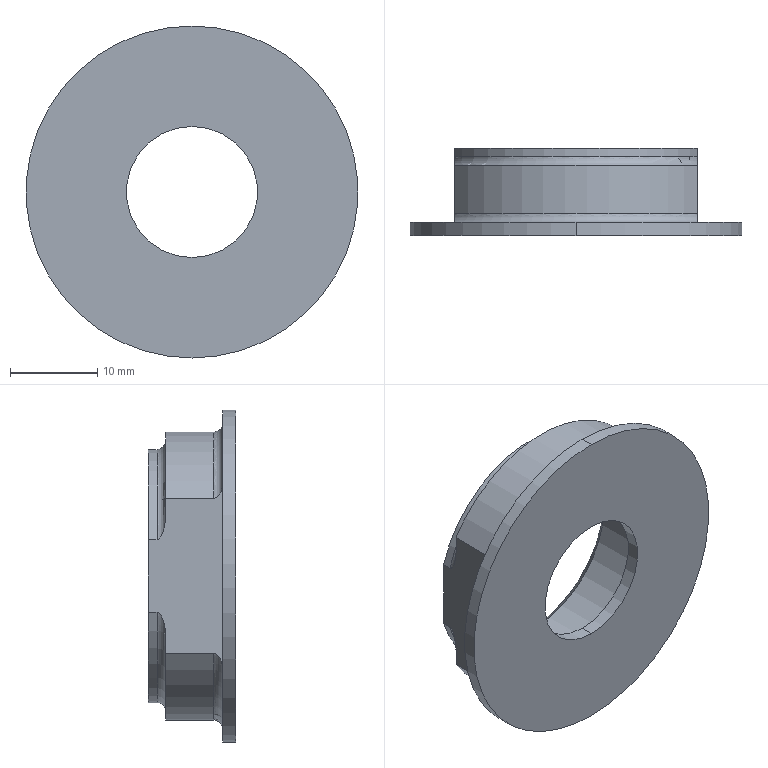Part | SolidWorks | features HoleWzd 1, ICE 1, Revolution 1 | 1 solid | 31 faces | box 38 x 10 x 38 mm | volume 4506 mm3 | cylinder 14 | plane 9 | torus 6 | cone 2 | commonest cylinder face diameters 29 x3 33 x3 15 x2 22 x2 26 x2 38 x2
STEP:
#1=CARTESIAN_POINT('',(0.,8.975,-11.));
#2=VERTEX_POINT('',#1);
#3=CARTESIAN_POINT('',(0.,8.975,11.));
#4=VERTEX_POINT('',#3);
#5=CARTESIAN_POINT('',(0.,8.975,0.));
#6=DIRECTION('',(0.,1.,0.));
#7=DIRECTION('',(0.,0.,1.));
#8=AXIS2_PLACEMENT_3D('',#5,#6,#7);
#9=CIRCLE('',#8,11.);
#10=EDGE_CURVE('',#2,#4,#9,.T.);
#11=ORIENTED_EDGE('',*,*,#10,.F.);
#12=CARTESIAN_POINT('',(0.,10.,-12.025));
#13=VERTEX_POINT('',#12);
#14=CARTESIAN_POINT('',(0.,10.,-12.025));
#15=DIRECTION('',(0.,0.7071,-0.7071));
#16=VECTOR('',#15,1000.);
#17=LINE('',#14,#16);
#18=EDGE_CURVE('',#2,#13,#17,.T.);
#19=ORIENTED_EDGE('',*,*,#18,.T.);
#20=CARTESIAN_POINT('',(0.,10.,12.025));
#21=VERTEX_POINT('',#20);
#22=CARTESIAN_POINT('',(0.,10.,0.));
#23=DIRECTION('',(0.,1.,0.));
#24=DIRECTION('',(0.,0.,1.));
#25=AXIS2_PLACEMENT_3D('',#22,#23,#24);
#26=CIRCLE('',#25,12.025);
#27=EDGE_CURVE('',#13,#21,#26,.T.);
#28=ORIENTED_EDGE('',*,*,#27,.T.);
#29=CARTESIAN_POINT('',(0.,10.,12.025));
#30=DIRECTION('',(0.,0.7071,0.7071));
#31=VECTOR('',#30,1000.);
#32=LINE('',#29,#31);
#33=EDGE_CURVE('',#4,#21,#32,.T.);
#34=ORIENTED_EDGE('',*,*,#33,.F.);
#35=EDGE_LOOP('',(#11,#19,#28,#34));
#36=FACE_OUTER_BOUND('',#35,.T.);
#37=CARTESIAN_POINT('',(0.,10.,0.));
#38=DIRECTION('',(0.,1.,0.));
#39=DIRECTION('',(0.,0.,1.));
#40=AXIS2_PLACEMENT_3D('',#37,#38,#39);
#41=CONICAL_SURFACE('',#40,12.025,0.7854);
#42=ADVANCED_FACE('',(#36),#41,.F.);
#43=CARTESIAN_POINT('',(0.,2.5,11.));
#44=VERTEX_POINT('',#43);
#45=CARTESIAN_POINT('',(0.,2.5,-11.));
#46=VERTEX_POINT('',#45);
#47=CARTESIAN_POINT('',(0.,2.5,0.));
#48=DIRECTION('',(0.,-1.,0.));
#49=DIRECTION('',(0.,0.,-1.));
#50=AXIS2_PLACEMENT_3D('',#47,#48,#49);
#51=CIRCLE('',#50,11.);
#52=EDGE_CURVE('',#44,#46,#51,.T.);
#53=ORIENTED_EDGE('',*,*,#52,.T.);
#54=CARTESIAN_POINT('',(0.,10.,-11.));
#55=DIRECTION('',(0.,1.,0.));
#56=VECTOR('',#55,1000.);
#57=LINE('',#54,#56);
#58=EDGE_CURVE('',#46,#2,#57,.T.);
#59=ORIENTED_EDGE('',*,*,#58,.T.);
#60=ORIENTED_EDGE('',*,*,#10,.T.);
#61=CARTESIAN_POINT('',(0.,10.,11.));
#62=DIRECTION('',(0.,1.,0.));
#63=VECTOR('',#62,1000.);
#64=LINE('',#61,#63);
#65=EDGE_CURVE('',#44,#4,#64,.T.);
#66=ORIENTED_EDGE('',*,*,#65,.F.);
#67=EDGE_LOOP('',(#53,#59,#60,#66));
#68=FACE_OUTER_BOUND('',#67,.T.);
#69=CARTESIAN_POINT('',(0.,10.,0.));
#70=DIRECTION('',(0.,1.,0.));
#71=DIRECTION('',(0.,0.,1.));
#72=AXIS2_PLACEMENT_3D('',#69,#70,#71);
#73=CYLINDRICAL_SURFACE('',#72,11.);
#74=ADVANCED_FACE('',(#68),#73,.F.);
#75=CARTESIAN_POINT('',(0.,1.5,-19.));
#76=VERTEX_POINT('',#75);
#77=CARTESIAN_POINT('',(0.,1.5,19.));
#78=VERTEX_POINT('',#77);
#79=CARTESIAN_POINT('',(0.,1.5,0.));
#80=DIRECTION('',(0.,-1.,0.));
#81=DIRECTION('',(0.,0.,-1.));
#82=AXIS2_PLACEMENT_3D('',#79,#80,#81);
#83=CIRCLE('',#82,19.);
#84=EDGE_CURVE('',#76,#78,#83,.T.);
#85=ORIENTED_EDGE('',*,*,#84,.T.);
#86=CARTESIAN_POINT('',(0.,0.,19.));
#87=VERTEX_POINT('',#86);
#88=CARTESIAN_POINT('',(0.,0.,19.));
#89=DIRECTION('',(0.,-1.,0.));
#90=VECTOR('',#89,1000.);
#91=LINE('',#88,#90);
#92=EDGE_CURVE('',#78,#87,#91,.T.);
#93=ORIENTED_EDGE('',*,*,#92,.T.);
#94=CARTESIAN_POINT('',(0.,0.,-19.));
#95=VERTEX_POINT('',#94);
#96=CARTESIAN_POINT('',(0.,0.,0.));
#97=DIRECTION('',(0.,-1.,0.));
#98=DIRECTION('',(0.,0.,-1.));
#99=AXIS2_PLACEMENT_3D('',#96,#97,#98);
#100=CIRCLE('',#99,19.);
#101=EDGE_CURVE('',#95,#87,#100,.T.);
#102=ORIENTED_EDGE('',*,*,#101,.F.);
#103=CARTESIAN_POINT('',(0.,0.,-19.));
#104=DIRECTION('',(0.,-1.,0.));
#105=VECTOR('',#104,1000.);
#106=LINE('',#103,#105);
#107=EDGE_CURVE('',#76,#95,#106,.T.);
#108=ORIENTED_EDGE('',*,*,#107,.F.);
#109=EDGE_LOOP('',(#85,#93,#102,#108));
#110=FACE_OUTER_BOUND('',#109,.T.);
#111=CARTESIAN_POINT('',(0.,0.,0.));
#112=DIRECTION('',(0.,-1.,0.));
#113=DIRECTION('',(0.,0.,-1.));
#114=AXIS2_PLACEMENT_3D('',#111,#112,#113);
#115=CYLINDRICAL_SURFACE('',#114,19.);
#116=ADVANCED_FACE('',(#110),#115,.T.);
#117=CARTESIAN_POINT('',(0.,2.5,13.));
#118=VERTEX_POINT('',#117);
#119=CARTESIAN_POINT('',(0.,2.5,-13.));
#120=VERTEX_POINT('',#119);
#121=CARTESIAN_POINT('',(0.,2.5,0.));
#122=DIRECTION('',(0.,-1.,0.));
#123=DIRECTION('',(0.,0.,-1.));
#124=AXIS2_PLACEMENT_3D('',#121,#122,#123);
#125=CIRCLE('',#124,13.);
#126=EDGE_CURVE('',#118,#120,#125,.T.);
#127=ORIENTED_EDGE('',*,*,#126,.F.);
#128=CARTESIAN_POINT('',(0.,1.5,13.));
#129=VERTEX_POINT('',#128);
#130=CARTESIAN_POINT('',(0.,0.,13.));
#131=DIRECTION('',(0.,-1.,0.));
#132=VECTOR('',#131,1000.);
#133=LINE('',#130,#132);
#134=EDGE_CURVE('',#118,#129,#133,.T.);
#135=ORIENTED_EDGE('',*,*,#134,.T.);
#136=CARTESIAN_POINT('',(0.,1.5,-13.));
#137=VERTEX_POINT('',#136);
#138=CARTESIAN_POINT('',(0.,1.5,0.));
#139=DIRECTION('',(0.,-1.,0.));
#140=DIRECTION('',(0.,0.,-1.));
#141=AXIS2_PLACEMENT_3D('',#138,#139,#140);
#142=CIRCLE('',#141,13.);
#143=EDGE_CURVE('',#129,#137,#142,.T.);
#144=ORIENTED_EDGE('',*,*,#143,.T.);
#145=CARTESIAN_POINT('',(0.,0.,-13.));
#146=DIRECTION('',(0.,-1.,0.));
#147=VECTOR('',#146,1000.);
#148=LINE('',#145,#147);
#149=EDGE_CURVE('',#120,#137,#148,.T.);
#150=ORIENTED_EDGE('',*,*,#149,.F.);
#151=EDGE_LOOP('',(#127,#135,#144,#150));
#152=FACE_OUTER_BOUND('',#151,.T.);
#153=CARTESIAN_POINT('',(0.,0.,0.));
#154=DIRECTION('',(0.,-1.,0.));
#155=DIRECTION('',(0.,0.,-1.));
#156=AXIS2_PLACEMENT_3D('',#153,#154,#155);
#157=CYLINDRICAL_SURFACE('',#156,13.);
#158=ADVANCED_FACE('',(#152),#157,.F.);
#159=CARTESIAN_POINT('',(0.,1.5,7.5));
#160=VERTEX_POINT('',#159);
#161=CARTESIAN_POINT('',(0.,1.5,-7.5));
#162=VERTEX_POINT('',#161);
#163=CARTESIAN_POINT('',(0.,1.5,0.));
#164=DIRECTION('',(0.,-1.,0.));
#165=DIRECTION('',(0.,0.,-1.));
#166=AXIS2_PLACEMENT_3D('',#163,#164,#165);
#167=CIRCLE('',#166,7.5);
#168=EDGE_CURVE('',#160,#162,#167,.T.);
#169=ORIENTED_EDGE('',*,*,#168,.F.);
#170=CARTESIAN_POINT('',(0.,0.,7.5));
#171=VERTEX_POINT('',#170);
#172=CARTESIAN_POINT('',(0.,0.,7.5));
#173=DIRECTION('',(0.,-1.,0.));
#174=VECTOR('',#173,1000.);
#175=LINE('',#172,#174);
#176=EDGE_CURVE('',#160,#171,#175,.T.);
#177=ORIENTED_EDGE('',*,*,#176,.T.);
#178=CARTESIAN_POINT('',(0.,0.,-7.5));
#179=VERTEX_POINT('',#178);
#180=CARTESIAN_POINT('',(0.,0.,0.));
#181=DIRECTION('',(0.,-1.,0.));
#182=DIRECTION('',(0.,0.,-1.));
#183=AXIS2_PLACEMENT_3D('',#180,#181,#182);
#184=CIRCLE('',#183,7.5);
#185=EDGE_CURVE('',#171,#179,#184,.T.);
#186=ORIENTED_EDGE('',*,*,#185,.T.);
#187=CARTESIAN_POINT('',(0.,0.,-7.5));
#188=DIRECTION('',(0.,-1.,0.));
#189=VECTOR('',#188,1000.);
#190=LINE('',#187,#189);
#191=EDGE_CURVE('',#162,#179,#190,.T.);
#192=ORIENTED_EDGE('',*,*,#191,.F.);
#193=EDGE_LOOP('',(#169,#177,#186,#192));
#194=FACE_OUTER_BOUND('',#193,.T.);
#195=CARTESIAN_POINT('',(0.,0.,0.));
#196=DIRECTION('',(0.,-1.,0.));
#197=DIRECTION('',(0.,0.,-1.));
#198=AXIS2_PLACEMENT_3D('',#195,#196,#197);
#199=CYLINDRICAL_SURFACE('',#198,7.5);
#200=ADVANCED_FACE('',(#194),#199,.F.);
#201=CARTESIAN_POINT('',(0.,1.5,-17.5));
#202=VERTEX_POINT('',#201);
#203=CARTESIAN_POINT('',(13.9,1.5,-10.632));
#204=VERTEX_POINT('',#203);
#205=CARTESIAN_POINT('',(0.,1.5,0.));
#206=DIRECTION('',(0.,-1.,0.));
#207=DIRECTION('',(0.,0.,-1.));
#208=AXIS2_PLACEMENT_3D('',#205,#206,#207);
#209=CIRCLE('',#208,17.5);
#210=EDGE_CURVE('',#202,#204,#209,.T.);
#211=ORIENTED_EDGE('',*,*,#210,.F.);
#212=CARTESIAN_POINT('',(0.,2.5,-16.5));
#213=VERTEX_POINT('',#212);
#214=CARTESIAN_POINT('',(0.,2.5,-17.5));
#215=DIRECTION('',(-1.,0.,0.));
#216=DIRECTION('',(0.,0.,1.));
#217=AXIS2_PLACEMENT_3D('',#214,#215,#216);
#218=CIRCLE('',#217,1.);
#219=EDGE_CURVE('',#202,#213,#218,.T.);
#220=ORIENTED_EDGE('',*,*,#219,.T.);
#221=CARTESIAN_POINT('',(13.9,2.5,-8.89));
#222=VERTEX_POINT('',#221);
#223=CARTESIAN_POINT('',(0.,2.5,0.));
#224=DIRECTION('',(0.,-1.,0.));
#225=DIRECTION('',(0.,0.,-1.));
#226=AXIS2_PLACEMENT_3D('',#223,#224,#225);
#227=CIRCLE('',#226,16.5);
#228=EDGE_CURVE('',#213,#222,#227,.T.);
#229=ORIENTED_EDGE('',*,*,#228,.T.);
#230=CARTESIAN_POINT('',(13.9,2.5,-8.89));
#231=CARTESIAN_POINT('',(13.9,2.408,-8.89));
#232=CARTESIAN_POINT('',(13.9,2.318,-8.915));
#233=CARTESIAN_POINT('',(13.9,2.154,-8.998));
#234=CARTESIAN_POINT('',(13.9,2.081,-9.055));
#235=CARTESIAN_POINT('',(13.9,1.952,-9.184));
#236=CARTESIAN_POINT('',(13.9,1.896,-9.257));
#237=CARTESIAN_POINT('',(13.9,1.797,-9.41));
#238=CARTESIAN_POINT('',(13.9,1.755,-9.49));
#239=CARTESIAN_POINT('',(13.9,1.642,-9.739));
#240=CARTESIAN_POINT('',(13.9,1.589,-9.914));
#241=CARTESIAN_POINT('',(13.9,1.518,-10.268));
#242=CARTESIAN_POINT('',(13.9,1.5,-10.451));
#243=CARTESIAN_POINT('',(13.9,1.5,-10.632));
#244=B_SPLINE_CURVE_WITH_KNOTS('',3,(#230,#231,#232,#233,#234,#235,#236,#237,#238,#239,#240,#241,#242,#243),.UNSPECIFIED.,.F.,.F.,(4,2,2,2,2,2,4),(0.004753,0.005027,0.005301,0.005575,0.005849,0.006397,0.006945),.UNSPECIFIED.);
#245=EDGE_CURVE('',#222,#204,#244,.T.);
#246=ORIENTED_EDGE('',*,*,#245,.T.);
#247=EDGE_LOOP('',(#211,#220,#229,#246));
#248=FACE_OUTER_BOUND('',#247,.T.);
#249=CARTESIAN_POINT('',(0.,2.5,0.));
#250=DIRECTION('',(0.,-1.,0.));
#251=DIRECTION('',(0.,0.,-1.));
#252=AXIS2_PLACEMENT_3D('',#249,#250,#251);
#253=TOROIDAL_SURFACE('',#252,17.5,1.);
#254=ADVANCED_FACE('',(#248),#253,.F.);
#255=CARTESIAN_POINT('',(-13.9,8.,-8.89));
#256=VERTEX_POINT('',#255);
#257=CARTESIAN_POINT('',(0.,8.,-16.5));
#258=VERTEX_POINT('',#257);
#259=CARTESIAN_POINT('',(0.,8.,0.));
#260=DIRECTION('',(0.,-1.,0.));
#261=DIRECTION('',(0.,0.,-1.));
#262=AXIS2_PLACEMENT_3D('',#259,#260,#261);
#263=CIRCLE('',#262,16.5);
#264=EDGE_CURVE('',#256,#258,#263,.T.);
#265=ORIENTED_EDGE('',*,*,#264,.T.);
#266=CARTESIAN_POINT('',(0.,0.,-16.5));
#267=DIRECTION('',(0.,-1.,0.));
#268=VECTOR('',#267,1000.);
#269=LINE('',#266,#268);
#270=EDGE_CURVE('',#258,#213,#269,.T.);
#271=ORIENTED_EDGE('',*,*,#270,.T.);
#272=CARTESIAN_POINT('',(-13.9,2.5,-8.89));
#273=VERTEX_POINT('',#272);
#274=CARTESIAN_POINT('',(0.,2.5,0.));
#275=DIRECTION('',(0.,-1.,0.));
#276=DIRECTION('',(0.,0.,-1.));
#277=AXIS2_PLACEMENT_3D('',#274,#275,#276);
#278=CIRCLE('',#277,16.5);
#279=EDGE_CURVE('',#273,#213,#278,.T.);
#280=ORIENTED_EDGE('',*,*,#279,.F.);
#281=CARTESIAN_POINT('',(-13.9,0.,-8.89));
#282=DIRECTION('',(0.,1.,0.));
#283=VECTOR('',#282,1000.);
#284=LINE('',#281,#283);
#285=EDGE_CURVE('',#273,#256,#284,.T.);
#286=ORIENTED_EDGE('',*,*,#285,.T.);
#287=EDGE_LOOP('',(#265,#271,#280,#286));
#288=FACE_OUTER_BOUND('',#287,.T.);
#289=CARTESIAN_POINT('',(0.,0.,0.));
#290=DIRECTION('',(0.,-1.,0.));
#291=DIRECTION('',(0.,0.,-1.));
#292=AXIS2_PLACEMENT_3D('',#289,#290,#291);
#293=CYLINDRICAL_SURFACE('',#292,16.5);
#294=ADVANCED_FACE('',(#288),#293,.T.);
#295=CARTESIAN_POINT('',(0.,8.,-15.5));
#296=VERTEX_POINT('',#295);
#297=CARTESIAN_POINT('',(13.9,8.,-6.859));
#298=VERTEX_POINT('',#297);
#299=CARTESIAN_POINT('',(0.,8.,0.));
#300=DIRECTION('',(0.,-1.,0.));
#301=DIRECTION('',(0.,0.,-1.));
#302=AXIS2_PLACEMENT_3D('',#299,#300,#301);
#303=CIRCLE('',#302,15.5);
#304=EDGE_CURVE('',#296,#298,#303,.T.);
#305=ORIENTED_EDGE('',*,*,#304,.F.);
#306=CARTESIAN_POINT('',(0.,9.,-14.5));
#307=VERTEX_POINT('',#306);
#308=CARTESIAN_POINT('',(0.,9.,-15.5));
#309=DIRECTION('',(-1.,0.,0.));
#310=DIRECTION('',(0.,0.,1.));
#311=AXIS2_PLACEMENT_3D('',#308,#309,#310);
#312=CIRCLE('',#311,1.);
#313=EDGE_CURVE('',#296,#307,#312,.T.);
#314=ORIENTED_EDGE('',*,*,#313,.T.);
#315=CARTESIAN_POINT('',(13.9,9.,-4.128));
#316=VERTEX_POINT('',#315);
#317=CARTESIAN_POINT('',(0.,9.,0.));
#318=DIRECTION('',(0.,-1.,0.));
#319=DIRECTION('',(0.,0.,-1.));
#320=AXIS2_PLACEMENT_3D('',#317,#318,#319);
#321=CIRCLE('',#320,14.5);
#322=EDGE_CURVE('',#307,#316,#321,.T.);
#323=ORIENTED_EDGE('',*,*,#322,.T.);
#324=CARTESIAN_POINT('',(13.9,9.,-4.128));
#325=CARTESIAN_POINT('',(13.9,8.936,-4.128));
#326=CARTESIAN_POINT('',(13.9,8.872,-4.152));
#327=CARTESIAN_POINT('',(13.9,8.763,-4.222));
#328=CARTESIAN_POINT('',(13.9,8.716,-4.267));
#329=CARTESIAN_POINT('',(13.9,8.59,-4.413));
#330=CARTESIAN_POINT('',(13.9,8.525,-4.523));
#331=CARTESIAN_POINT('',(13.9,8.352,-4.868));
#332=CARTESIAN_POINT('',(13.9,8.271,-5.108));
#333=CARTESIAN_POINT('',(13.9,8.137,-5.597));
#334=CARTESIAN_POINT('',(13.9,8.087,-5.848));
#335=CARTESIAN_POINT('',(13.9,8.018,-6.352));
#336=CARTESIAN_POINT('',(13.9,8.,-6.605));
#337=CARTESIAN_POINT('',(13.9,8.,-6.859));
#338=B_SPLINE_CURVE_WITH_KNOTS('',3,(#324,#325,#326,#327,#328,#329,#330,#331,#332,#333,#334,#335,#336,#337),.UNSPECIFIED.,.F.,.F.,(4,2,2,2,2,2,4),(0.005884,0.006078,0.006271,0.006658,0.007432,0.008206,0.00898),.UNSPECIFIED.);
#339=EDGE_CURVE('',#316,#298,#338,.T.);
#340=ORIENTED_EDGE('',*,*,#339,.T.);
#341=EDGE_LOOP('',(#305,#314,#323,#340));
#342=FACE_OUTER_BOUND('',#341,.T.);
#343=CARTESIAN_POINT('',(0.,9.,0.));
#344=DIRECTION('',(0.,-1.,0.));
#345=DIRECTION('',(0.,0.,-1.));
#346=AXIS2_PLACEMENT_3D('',#343,#344,#345);
#347=TOROIDAL_SURFACE('',#346,15.5,1.);
#348=ADVANCED_FACE('',(#342),#347,.F.);
#349=CARTESIAN_POINT('',(-13.9,10.,-4.128));
#350=VERTEX_POINT('',#349);
#351=CARTESIAN_POINT('',(0.,10.,-14.5));
#352=VERTEX_POINT('',#351);
#353=CARTESIAN_POINT('',(0.,10.,0.));
#354=DIRECTION('',(0.,-1.,0.));
#355=DIRECTION('',(0.,0.,-1.));
#356=AXIS2_PLACEMENT_3D('',#353,#354,#355);
#357=CIRCLE('',#356,14.5);
#358=EDGE_CURVE('',#350,#352,#357,.T.);
#359=ORIENTED_EDGE('',*,*,#358,.T.);
#360=CARTESIAN_POINT('',(0.,0.,-14.5));
#361=DIRECTION('',(0.,-1.,0.));
#362=VECTOR('',#361,1000.);
#363=LINE('',#360,#362);
#364=EDGE_CURVE('',#352,#307,#363,.T.);
#365=ORIENTED_EDGE('',*,*,#364,.T.);
#366=CARTESIAN_POINT('',(-13.9,9.,-4.128));
#367=VERTEX_POINT('',#366);
#368=CARTESIAN_POINT('',(0.,9.,0.));
#369=DIRECTION('',(0.,-1.,0.));
#370=DIRECTION('',(0.,0.,-1.));
#371=AXIS2_PLACEMENT_3D('',#368,#369,#370);
#372=CIRCLE('',#371,14.5);
#373=EDGE_CURVE('',#367,#307,#372,.T.);
#374=ORIENTED_EDGE('',*,*,#373,.F.);
#375=CARTESIAN_POINT('',(-13.9,0.,-4.128));
#376=DIRECTION('',(0.,1.,0.));
#377=VECTOR('',#376,1000.);
#378=LINE('',#375,#377);
#379=EDGE_CURVE('',#367,#350,#378,.T.);
#380=ORIENTED_EDGE('',*,*,#379,.T.);
#381=EDGE_LOOP('',(#359,#365,#374,#380));
#382=FACE_OUTER_BOUND('',#381,.T.);
#383=CARTESIAN_POINT('',(0.,0.,0.));
#384=DIRECTION('',(0.,-1.,0.));
#385=DIRECTION('',(0.,0.,-1.));
#386=AXIS2_PLACEMENT_3D('',#383,#384,#385);
#387=CYLINDRICAL_SURFACE('',#386,14.5);
#388=ADVANCED_FACE('',(#382),#387,.T.);
#389=CARTESIAN_POINT('',(0.,10.,0.));
#390=DIRECTION('',(0.,1.,0.));
#391=DIRECTION('',(0.,0.,1.));
#392=AXIS2_PLACEMENT_3D('',#389,#390,#391);
#393=CIRCLE('',#392,12.025);
#394=EDGE_CURVE('',#21,#13,#393,.T.);
#395=ORIENTED_EDGE('',*,*,#394,.F.);
#396=ORIENTED_EDGE('',*,*,#27,.F.);
#397=EDGE_LOOP('',(#395,#396));
#398=FACE_BOUND('',#397,.T.);
#399=ORIENTED_EDGE('',*,*,#358,.F.);
#400=CARTESIAN_POINT('',(-13.9,10.,4.128));
#401=VERTEX_POINT('',#400);
#402=CARTESIAN_POINT('',(-13.9,10.,-28.312));
#403=DIRECTION('',(0.,0.,1.));
#404=VECTOR('',#403,1000.);
#405=LINE('',#402,#404);
#406=EDGE_CURVE('',#350,#401,#405,.T.);
#407=ORIENTED_EDGE('',*,*,#406,.T.);
#408=CARTESIAN_POINT('',(13.9,10.,4.128));
#409=VERTEX_POINT('',#408);
#410=CARTESIAN_POINT('',(0.,10.,0.));
#411=DIRECTION('',(0.,-1.,0.));
#412=DIRECTION('',(0.,0.,-1.));
#413=AXIS2_PLACEMENT_3D('',#410,#411,#412);
#414=CIRCLE('',#413,14.5);
#415=EDGE_CURVE('',#409,#401,#414,.T.);
#416=ORIENTED_EDGE('',*,*,#415,.F.);
#417=CARTESIAN_POINT('',(13.9,10.,-4.128));
#418=VERTEX_POINT('',#417);
#419=CARTESIAN_POINT('',(13.9,10.,-28.312));
#420=DIRECTION('',(0.,0.,-1.));
#421=VECTOR('',#420,1000.);
#422=LINE('',#419,#421);
#423=EDGE_CURVE('',#409,#418,#422,.T.);
#424=ORIENTED_EDGE('',*,*,#423,.T.);
#425=CARTESIAN_POINT('',(0.,10.,0.));
#426=DIRECTION('',(0.,-1.,0.));
#427=DIRECTION('',(0.,0.,-1.));
#428=AXIS2_PLACEMENT_3D('',#425,#426,#427);
#429=CIRCLE('',#428,14.5);
#430=EDGE_CURVE('',#352,#418,#429,.T.);
#431=ORIENTED_EDGE('',*,*,#430,.F.);
#432=EDGE_LOOP('',(#399,#407,#416,#424,#431));
#433=FACE_OUTER_BOUND('',#432,.T.);
#434=CARTESIAN_POINT('',(14.5,10.,0.));
#435=DIRECTION('',(0.,1.,0.));
#436=DIRECTION('',(0.,0.,1.));
#437=AXIS2_PLACEMENT_3D('',#434,#435,#436);
#438=PLANE('',#437);
#439=ADVANCED_FACE('',(#398,#433),#438,.T.);
#440=ORIENTED_EDGE('',*,*,#364,.F.);
#441=ORIENTED_EDGE('',*,*,#430,.T.);
#442=CARTESIAN_POINT('',(13.9,0.,-4.128));
#443=DIRECTION('',(0.,-1.,0.));
#444=VECTOR('',#443,1000.);
#445=LINE('',#442,#444);
#446=EDGE_CURVE('',#418,#316,#445,.T.);
#447=ORIENTED_EDGE('',*,*,#446,.T.);
#448=ORIENTED_EDGE('',*,*,#322,.F.);
#449=EDGE_LOOP('',(#440,#441,#447,#448));
#450=FACE_OUTER_BOUND('',#449,.T.);
#451=CARTESIAN_POINT('',(0.,0.,0.));
#452=DIRECTION('',(0.,-1.,0.));
#453=DIRECTION('',(0.,0.,-1.));
#454=AXIS2_PLACEMENT_3D('',#451,#452,#453);
#455=CYLINDRICAL_SURFACE('',#454,14.5);
#456=ADVANCED_FACE('',(#450),#455,.T.);
#457=ORIENTED_EDGE('',*,*,#415,.T.);
#458=CARTESIAN_POINT('',(-13.9,9.,4.128));
#459=VERTEX_POINT('',#458);
#460=CARTESIAN_POINT('',(-13.9,0.,4.128));
#461=DIRECTION('',(0.,-1.,0.));
#462=VECTOR('',#461,1000.);
#463=LINE('',#460,#462);
#464=EDGE_CURVE('',#401,#459,#463,.T.);
#465=ORIENTED_EDGE('',*,*,#464,.T.);
#466=CARTESIAN_POINT('',(13.9,9.,4.128));
#467=VERTEX_POINT('',#466);
#468=CARTESIAN_POINT('',(0.,9.,0.));
#469=DIRECTION('',(0.,-1.,0.));
#470=DIRECTION('',(0.,0.,-1.));
#471=AXIS2_PLACEMENT_3D('',#468,#469,#470);
#472=CIRCLE('',#471,14.5);
#473=EDGE_CURVE('',#467,#459,#472,.T.);
#474=ORIENTED_EDGE('',*,*,#473,.F.);
#475=CARTESIAN_POINT('',(13.9,0.,4.128));
#476=DIRECTION('',(0.,1.,0.));
#477=VECTOR('',#476,1000.);
#478=LINE('',#475,#477);
#479=EDGE_CURVE('',#467,#409,#478,.T.);
#480=ORIENTED_EDGE('',*,*,#479,.T.);
#481=EDGE_LOOP('',(#457,#465,#474,#480));
#482=FACE_OUTER_BOUND('',#481,.T.);
#483=CARTESIAN_POINT('',(0.,0.,0.));
#484=DIRECTION('',(0.,-1.,0.));
#485=DIRECTION('',(0.,0.,-1.));
#486=AXIS2_PLACEMENT_3D('',#483,#484,#485);
#487=CYLINDRICAL_SURFACE('',#486,14.5);
#488=ADVANCED_FACE('',(#482),#487,.T.);
#489=ORIENTED_EDGE('',*,*,#313,.F.);
#490=CARTESIAN_POINT('',(-13.9,8.,-6.859));
#491=VERTEX_POINT('',#490);
#492=CARTESIAN_POINT('',(0.,8.,0.));
#493=DIRECTION('',(0.,-1.,0.));
#494=DIRECTION('',(0.,0.,-1.));
#495=AXIS2_PLACEMENT_3D('',#492,#493,#494);
#496=CIRCLE('',#495,15.5);
#497=EDGE_CURVE('',#491,#296,#496,.T.);
#498=ORIENTED_EDGE('',*,*,#497,.F.);
#499=CARTESIAN_POINT('',(-13.9,8.,-6.859));
#500=CARTESIAN_POINT('',(-13.9,8.,-6.604));
#501=CARTESIAN_POINT('',(-13.9,8.019,-6.352));
#502=CARTESIAN_POINT('',(-13.9,8.087,-5.851));
#503=CARTESIAN_POINT('',(-13.9,8.136,-5.602));
#504=CARTESIAN_POINT('',(-13.9,8.27,-5.109));
#505=CARTESIAN_POINT('',(-13.9,8.353,-4.867));
#506=CARTESIAN_POINT('',(-13.9,8.524,-4.526));
#507=CARTESIAN_POINT('',(-13.9,8.59,-4.414));
#508=CARTESIAN_POINT('',(-13.9,8.716,-4.267));
#509=CARTESIAN_POINT('',(-13.9,8.763,-4.221));
#510=CARTESIAN_POINT('',(-13.9,8.871,-4.152));
#511=CARTESIAN_POINT('',(-13.9,8.935,-4.128));
#512=CARTESIAN_POINT('',(-13.9,9.,-4.128));
#513=B_SPLINE_CURVE_WITH_KNOTS('',3,(#499,#500,#501,#502,#503,#504,#505,#506,#507,#508,#509,#510,#511,#512),.UNSPECIFIED.,.F.,.F.,(4,2,2,2,2,2,4),(0.002134,0.002899,0.003665,0.004431,0.004813,0.005005,0.005196),.UNSPECIFIED.);
#514=EDGE_CURVE('',#491,#367,#513,.T.);
#515=ORIENTED_EDGE('',*,*,#514,.T.);
#516=ORIENTED_EDGE('',*,*,#373,.T.);
#517=EDGE_LOOP('',(#489,#498,#515,#516));
#518=FACE_OUTER_BOUND('',#517,.T.);
#519=CARTESIAN_POINT('',(0.,9.,0.));
#520=DIRECTION('',(0.,-1.,0.));
#521=DIRECTION('',(0.,0.,-1.));
#522=AXIS2_PLACEMENT_3D('',#519,#520,#521);
#523=TOROIDAL_SURFACE('',#522,15.5,1.);
#524=ADVANCED_FACE('',(#518),#523,.F.);
#525=ORIENTED_EDGE('',*,*,#473,.T.);
#526=CARTESIAN_POINT('',(-13.9,8.,6.859));
#527=VERTEX_POINT('',#526);
#528=CARTESIAN_POINT('',(-13.9,9.,4.128));
#529=CARTESIAN_POINT('',(-13.9,8.935,4.128));
#530=CARTESIAN_POINT('',(-13.9,8.872,4.152));
#531=CARTESIAN_POINT('',(-13.9,8.764,4.221));
#532=CARTESIAN_POINT('',(-13.9,8.716,4.267));
#533=CARTESIAN_POINT('',(-13.9,8.591,4.413));
#534=CARTESIAN_POINT('',(-13.9,8.525,4.525));
#535=CARTESIAN_POINT('',(-13.9,8.353,4.866));
#536=CARTESIAN_POINT('',(-13.9,8.27,5.11));
#537=CARTESIAN_POINT('',(-13.9,8.136,5.602));
#538=CARTESIAN_POINT('',(-13.9,8.087,5.85));
#539=CARTESIAN_POINT('',(-13.9,8.019,6.351));
#540=CARTESIAN_POINT('',(-13.9,8.,6.604));
#541=CARTESIAN_POINT('',(-13.9,8.,6.859));
#542=B_SPLINE_CURVE_WITH_KNOTS('',3,(#528,#529,#530,#531,#532,#533,#534,#535,#536,#537,#538,#539,#540,#541),.UNSPECIFIED.,.F.,.F.,(4,2,2,2,2,2,4),(0.0000023,0.0001952,0.000388,0.0007737,0.001545,0.002317,0.003088),.UNSPECIFIED.);
#543=EDGE_CURVE('',#459,#527,#542,.T.);
#544=ORIENTED_EDGE('',*,*,#543,.T.);
#545=CARTESIAN_POINT('',(13.9,8.,6.859));
#546=VERTEX_POINT('',#545);
#547=CARTESIAN_POINT('',(0.,8.,0.));
#548=DIRECTION('',(0.,-1.,0.));
#549=DIRECTION('',(0.,0.,-1.));
#550=AXIS2_PLACEMENT_3D('',#547,#548,#549);
#551=CIRCLE('',#550,15.5);
#552=EDGE_CURVE('',#546,#527,#551,.T.);
#553=ORIENTED_EDGE('',*,*,#552,.F.);
#554=CARTESIAN_POINT('',(13.9,8.,6.859));
#555=CARTESIAN_POINT('',(13.9,8.,6.604));
#556=CARTESIAN_POINT('',(13.9,8.019,6.348));
#557=CARTESIAN_POINT('',(13.9,8.087,5.846));
#558=CARTESIAN_POINT('',(13.9,8.137,5.599));
#559=CARTESIAN_POINT('',(13.9,8.269,5.112));
#560=CARTESIAN_POINT('',(13.9,8.351,4.871));
#561=CARTESIAN_POINT('',(13.9,8.525,4.525));
#562=CARTESIAN_POINT('',(13.9,8.591,4.413));
#563=CARTESIAN_POINT('',(13.9,8.716,4.268));
#564=CARTESIAN_POINT('',(13.9,8.762,4.223));
#565=CARTESIAN_POINT('',(13.9,8.871,4.152));
#566=CARTESIAN_POINT('',(13.9,8.934,4.128));
#567=CARTESIAN_POINT('',(13.9,9.,4.128));
#568=B_SPLINE_CURVE_WITH_KNOTS('',3,(#554,#555,#556,#557,#558,#559,#560,#561,#562,#563,#564,#565,#566,#567),.UNSPECIFIED.,.F.,.F.,(4,2,2,2,2,2,4),(0.008027,0.008796,0.009565,0.01033,0.01072,0.01091,0.0111),.UNSPECIFIED.);
#569=EDGE_CURVE('',#546,#467,#568,.T.);
#570=ORIENTED_EDGE('',*,*,#569,.T.);
#571=EDGE_LOOP('',(#525,#544,#553,#570));
#572=FACE_OUTER_BOUND('',#571,.T.);
#573=CARTESIAN_POINT('',(0.,9.,0.));
#574=DIRECTION('',(0.,-1.,0.));
#575=DIRECTION('',(0.,0.,-1.));
#576=AXIS2_PLACEMENT_3D('',#573,#574,#575);
#577=TOROIDAL_SURFACE('',#576,15.5,1.);
#578=ADVANCED_FACE('',(#572),#577,.F.);
#579=ORIENTED_EDGE('',*,*,#264,.F.);
#580=CARTESIAN_POINT('',(-13.9,8.,0.));
#581=DIRECTION('',(0.,0.,1.));
#582=VECTOR('',#581,1000.);
#583=LINE('',#580,#582);
#584=EDGE_CURVE('',#256,#491,#583,.T.);
#585=ORIENTED_EDGE('',*,*,#584,.T.);
#586=ORIENTED_EDGE('',*,*,#497,.T.);
#587=ORIENTED_EDGE('',*,*,#304,.T.);
#588=CARTESIAN_POINT('',(13.9,8.,-8.89));
#589=VERTEX_POINT('',#588);
#590=CARTESIAN_POINT('',(13.9,8.,0.));
#591=DIRECTION('',(0.,0.,-1.));
#592=VECTOR('',#591,1000.);
#593=LINE('',#590,#592);
#594=EDGE_CURVE('',#298,#589,#593,.T.);
#595=ORIENTED_EDGE('',*,*,#594,.T.);
#596=CARTESIAN_POINT('',(0.,8.,0.));
#597=DIRECTION('',(0.,-1.,0.));
#598=DIRECTION('',(0.,0.,-1.));
#599=AXIS2_PLACEMENT_3D('',#596,#597,#598);
#600=CIRCLE('',#599,16.5);
#601=EDGE_CURVE('',#258,#589,#600,.T.);
#602=ORIENTED_EDGE('',*,*,#601,.F.);
#603=EDGE_LOOP('',(#579,#585,#586,#587,#595,#602));
#604=FACE_OUTER_BOUND('',#603,.T.);
#605=CARTESIAN_POINT('',(15.5,8.,0.));
#606=DIRECTION('',(0.,1.,0.));
#607=DIRECTION('',(0.,0.,1.));
#608=AXIS2_PLACEMENT_3D('',#605,#606,#607);
#609=PLANE('',#608);
#610=ADVANCED_FACE('',(#604),#609,.T.);
#611=ORIENTED_EDGE('',*,*,#552,.T.);
#612=CARTESIAN_POINT('',(-13.9,8.,8.89));
#613=VERTEX_POINT('',#612);
#614=CARTESIAN_POINT('',(-13.9,8.,0.));
#615=DIRECTION('',(0.,0.,1.));
#616=VECTOR('',#615,1000.);
#617=LINE('',#614,#616);
#618=EDGE_CURVE('',#527,#613,#617,.T.);
#619=ORIENTED_EDGE('',*,*,#618,.T.);
#620=CARTESIAN_POINT('',(13.9,8.,8.89));
#621=VERTEX_POINT('',#620);
#622=CARTESIAN_POINT('',(0.,8.,0.));
#623=DIRECTION('',(0.,-1.,0.));
#624=DIRECTION('',(0.,0.,-1.));
#625=AXIS2_PLACEMENT_3D('',#622,#623,#624);
#626=CIRCLE('',#625,16.5);
#627=EDGE_CURVE('',#621,#613,#626,.T.);
#628=ORIENTED_EDGE('',*,*,#627,.F.);
#629=CARTESIAN_POINT('',(13.9,8.,0.));
#630=DIRECTION('',(0.,0.,-1.));
#631=VECTOR('',#630,1000.);
#632=LINE('',#629,#631);
#633=EDGE_CURVE('',#621,#546,#632,.T.);
#634=ORIENTED_EDGE('',*,*,#633,.T.);
#635=EDGE_LOOP('',(#611,#619,#628,#634));
#636=FACE_OUTER_BOUND('',#635,.T.);
#637=CARTESIAN_POINT('',(15.5,8.,0.));
#638=DIRECTION('',(0.,1.,0.));
#639=DIRECTION('',(0.,0.,1.));
#640=AXIS2_PLACEMENT_3D('',#637,#638,#639);
#641=PLANE('',#640);
#642=ADVANCED_FACE('',(#636),#641,.T.);
#643=ORIENTED_EDGE('',*,*,#270,.F.);
#644=ORIENTED_EDGE('',*,*,#601,.T.);
#645=CARTESIAN_POINT('',(13.9,0.,-8.89));
#646=DIRECTION('',(0.,-1.,0.));
#647=VECTOR('',#646,1000.);
#648=LINE('',#645,#647);
#649=EDGE_CURVE('',#589,#222,#648,.T.);
#650=ORIENTED_EDGE('',*,*,#649,.T.);
#651=ORIENTED_EDGE('',*,*,#228,.F.);
#652=EDGE_LOOP('',(#643,#644,#650,#651));
#653=FACE_OUTER_BOUND('',#652,.T.);
#654=CARTESIAN_POINT('',(0.,0.,0.));
#655=DIRECTION('',(0.,-1.,0.));
#656=DIRECTION('',(0.,0.,-1.));
#657=AXIS2_PLACEMENT_3D('',#654,#655,#656);
#658=CYLINDRICAL_SURFACE('',#657,16.5);
#659=ADVANCED_FACE('',(#653),#658,.T.);
#660=ORIENTED_EDGE('',*,*,#627,.T.);
#661=CARTESIAN_POINT('',(-13.9,2.5,8.89));
#662=VERTEX_POINT('',#661);
#663=CARTESIAN_POINT('',(-13.9,0.,8.89));
#664=DIRECTION('',(0.,-1.,0.));
#665=VECTOR('',#664,1000.);
#666=LINE('',#663,#665);
#667=EDGE_CURVE('',#613,#662,#666,.T.);
#668=ORIENTED_EDGE('',*,*,#667,.T.);
#669=CARTESIAN_POINT('',(13.9,2.5,8.89));
#670=VERTEX_POINT('',#669);
#671=CARTESIAN_POINT('',(0.,2.5,0.));
#672=DIRECTION('',(0.,-1.,0.));
#673=DIRECTION('',(0.,0.,-1.));
#674=AXIS2_PLACEMENT_3D('',#671,#672,#673);
#675=CIRCLE('',#674,16.5);
#676=EDGE_CURVE('',#670,#662,#675,.T.);
#677=ORIENTED_EDGE('',*,*,#676,.F.);
#678=CARTESIAN_POINT('',(13.9,0.,8.89));
#679=DIRECTION('',(0.,1.,0.));
#680=VECTOR('',#679,1000.);
#681=LINE('',#678,#680);
#682=EDGE_CURVE('',#670,#621,#681,.T.);
#683=ORIENTED_EDGE('',*,*,#682,.T.);
#684=EDGE_LOOP('',(#660,#668,#677,#683));
#685=FACE_OUTER_BOUND('',#684,.T.);
#686=CARTESIAN_POINT('',(0.,0.,0.));
#687=DIRECTION('',(0.,-1.,0.));
#688=DIRECTION('',(0.,0.,-1.));
#689=AXIS2_PLACEMENT_3D('',#686,#687,#688);
#690=CYLINDRICAL_SURFACE('',#689,16.5);
#691=ADVANCED_FACE('',(#685),#690,.T.);
#692=ORIENTED_EDGE('',*,*,#219,.F.);
#693=CARTESIAN_POINT('',(-13.9,1.5,-10.632));
#694=VERTEX_POINT('',#693);
#695=CARTESIAN_POINT('',(0.,1.5,0.));
#696=DIRECTION('',(0.,-1.,0.));
#697=DIRECTION('',(0.,0.,-1.));
#698=AXIS2_PLACEMENT_3D('',#695,#696,#697);
#699=CIRCLE('',#698,17.5);
#700=EDGE_CURVE('',#694,#202,#699,.T.);
#701=ORIENTED_EDGE('',*,*,#700,.F.);
#702=CARTESIAN_POINT('',(-13.9,1.5,-10.632));
#703=CARTESIAN_POINT('',(-13.9,1.5,-10.451));
#704=CARTESIAN_POINT('',(-13.9,1.518,-10.268));
#705=CARTESIAN_POINT('',(-13.9,1.589,-9.913));
#706=CARTESIAN_POINT('',(-13.9,1.642,-9.741));
#707=CARTESIAN_POINT('',(-13.9,1.791,-9.408));
#708=CARTESIAN_POINT('',(-13.9,1.889,-9.248));
#709=CARTESIAN_POINT('',(-13.9,2.081,-9.055));
#710=CARTESIAN_POINT('',(-13.9,2.153,-8.998));
#711=CARTESIAN_POINT('',(-13.9,2.318,-8.915));
#712=CARTESIAN_POINT('',(-13.9,2.409,-8.89));
#713=CARTESIAN_POINT('',(-13.9,2.5,-8.89));
#714=B_SPLINE_CURVE_WITH_KNOTS('',3,(#702,#703,#704,#705,#706,#707,#708,#709,#710,#711,#712,#713),.UNSPECIFIED.,.F.,.F.,(4,2,2,2,2,4),(0.001543,0.002087,0.002631,0.003175,0.003447,0.003719),.UNSPECIFIED.);
#715=EDGE_CURVE('',#694,#273,#714,.T.);
#716=ORIENTED_EDGE('',*,*,#715,.T.);
#717=ORIENTED_EDGE('',*,*,#279,.T.);
#718=EDGE_LOOP('',(#692,#701,#716,#717));
#719=FACE_OUTER_BOUND('',#718,.T.);
#720=CARTESIAN_POINT('',(0.,2.5,0.));
#721=DIRECTION('',(0.,-1.,0.));
#722=DIRECTION('',(0.,0.,-1.));
#723=AXIS2_PLACEMENT_3D('',#720,#721,#722);
#724=TOROIDAL_SURFACE('',#723,17.5,1.);
#725=ADVANCED_FACE('',(#719),#724,.F.);
#726=ORIENTED_EDGE('',*,*,#676,.T.);
#727=CARTESIAN_POINT('',(-13.9,1.5,10.632));
#728=VERTEX_POINT('',#727);
#729=CARTESIAN_POINT('',(-13.9,2.5,8.89));
#730=CARTESIAN_POINT('',(-13.9,2.408,8.89));
#731=CARTESIAN_POINT('',(-13.9,2.318,8.915));
#732=CARTESIAN_POINT('',(-13.9,2.154,8.998));
#733=CARTESIAN_POINT('',(-13.9,2.081,9.055));
#734=CARTESIAN_POINT('',(-13.9,1.888,9.249));
#735=CARTESIAN_POINT('',(-13.9,1.792,9.407));
#736=CARTESIAN_POINT('',(-13.9,1.642,9.74));
#737=CARTESIAN_POINT('',(-13.9,1.589,9.913));
#738=CARTESIAN_POINT('',(-13.9,1.518,10.268));
#739=CARTESIAN_POINT('',(-13.9,1.5,10.451));
#740=CARTESIAN_POINT('',(-13.9,1.5,10.632));
#741=B_SPLINE_CURVE_WITH_KNOTS('',3,(#729,#730,#731,#732,#733,#734,#735,#736,#737,#738,#739,#740),.UNSPECIFIED.,.F.,.F.,(4,2,2,2,2,4),(0.008397,0.00867,0.008943,0.00949,0.01004,0.01058),.UNSPECIFIED.);
#742=EDGE_CURVE('',#662,#728,#741,.T.);
#743=ORIENTED_EDGE('',*,*,#742,.T.);
#744=CARTESIAN_POINT('',(13.9,1.5,10.632));
#745=VERTEX_POINT('',#744);
#746=CARTESIAN_POINT('',(0.,1.5,0.));
#747=DIRECTION('',(0.,-1.,0.));
#748=DIRECTION('',(0.,0.,-1.));
#749=AXIS2_PLACEMENT_3D('',#746,#747,#748);
#750=CIRCLE('',#749,17.5);
#751=EDGE_CURVE('',#745,#728,#750,.T.);
#752=ORIENTED_EDGE('',*,*,#751,.F.);
#753=CARTESIAN_POINT('',(13.9,1.5,10.632));
#754=CARTESIAN_POINT('',(13.9,1.5,10.45));
#755=CARTESIAN_POINT('',(13.9,1.518,10.268));
#756=CARTESIAN_POINT('',(13.9,1.589,9.914));
#757=CARTESIAN_POINT('',(13.9,1.643,9.739));
#758=CARTESIAN_POINT('',(13.9,1.792,9.407));
#759=CARTESIAN_POINT('',(13.9,1.889,9.248));
#760=CARTESIAN_POINT('',(13.9,2.081,9.055));
#761=CARTESIAN_POINT('',(13.9,2.154,8.998));
#762=CARTESIAN_POINT('',(13.9,2.317,8.915));
#763=CARTESIAN_POINT('',(13.9,2.409,8.89));
#764=CARTESIAN_POINT('',(13.9,2.5,8.89));
#765=B_SPLINE_CURVE_WITH_KNOTS('',3,(#753,#754,#755,#756,#757,#758,#759,#760,#761,#762,#763,#764),.UNSPECIFIED.,.F.,.F.,(4,2,2,2,2,4),(0.00637,0.006915,0.007459,0.008004,0.008276,0.008548),.UNSPECIFIED.);
#766=EDGE_CURVE('',#745,#670,#765,.T.);
#767=ORIENTED_EDGE('',*,*,#766,.T.);
#768=EDGE_LOOP('',(#726,#743,#752,#767));
#769=FACE_OUTER_BOUND('',#768,.T.);
#770=CARTESIAN_POINT('',(0.,2.5,0.));
#771=DIRECTION('',(0.,-1.,0.));
#772=DIRECTION('',(0.,0.,-1.));
#773=AXIS2_PLACEMENT_3D('',#770,#771,#772);
#774=TOROIDAL_SURFACE('',#773,17.5,1.);
#775=ADVANCED_FACE('',(#769),#774,.F.);
#776=ORIENTED_EDGE('',*,*,#176,.F.);
#777=CARTESIAN_POINT('',(0.,1.5,0.));
#778=DIRECTION('',(0.,-1.,0.));
#779=DIRECTION('',(0.,0.,-1.));
#780=AXIS2_PLACEMENT_3D('',#777,#778,#779);
#781=CIRCLE('',#780,7.5);
#782=EDGE_CURVE('',#162,#160,#781,.T.);
#783=ORIENTED_EDGE('',*,*,#782,.F.);
#784=ORIENTED_EDGE('',*,*,#191,.T.);
#785=CARTESIAN_POINT('',(0.,0.,0.));
#786=DIRECTION('',(0.,-1.,0.));
#787=DIRECTION('',(0.,0.,-1.));
#788=AXIS2_PLACEMENT_3D('',#785,#786,#787);
#789=CIRCLE('',#788,7.5);
#790=EDGE_CURVE('',#179,#171,#789,.T.);
#791=ORIENTED_EDGE('',*,*,#790,.T.);
#792=EDGE_LOOP('',(#776,#783,#784,#791));
#793=FACE_OUTER_BOUND('',#792,.T.);
#794=CARTESIAN_POINT('',(0.,0.,0.));
#795=DIRECTION('',(0.,-1.,0.));
#796=DIRECTION('',(0.,0.,-1.));
#797=AXIS2_PLACEMENT_3D('',#794,#795,#796);
#798=CYLINDRICAL_SURFACE('',#797,7.5);
#799=ADVANCED_FACE('',(#793),#798,.F.);
#800=ORIENTED_EDGE('',*,*,#782,.T.);
#801=ORIENTED_EDGE('',*,*,#168,.T.);
#802=EDGE_LOOP('',(#800,#801));
#803=FACE_BOUND('',#802,.T.);
#804=CARTESIAN_POINT('',(0.,1.5,0.));
#805=DIRECTION('',(0.,-1.,0.));
#806=DIRECTION('',(0.,0.,-1.));
#807=AXIS2_PLACEMENT_3D('',#804,#805,#806);
#808=CIRCLE('',#807,13.);
#809=EDGE_CURVE('',#137,#129,#808,.T.);
#810=ORIENTED_EDGE('',*,*,#809,.F.);
#811=ORIENTED_EDGE('',*,*,#143,.F.);
#812=EDGE_LOOP('',(#810,#811));
#813=FACE_OUTER_BOUND('',#812,.T.);
#814=CARTESIAN_POINT('',(13.,1.5,0.));
#815=DIRECTION('',(0.,1.,0.));
#816=DIRECTION('',(0.,0.,1.));
#817=AXIS2_PLACEMENT_3D('',#814,#815,#816);
#818=PLANE('',#817);
#819=ADVANCED_FACE('',(#803,#813),#818,.T.);
#820=ORIENTED_EDGE('',*,*,#134,.F.);
#821=CARTESIAN_POINT('',(0.,2.5,0.));
#822=DIRECTION('',(0.,-1.,0.));
#823=DIRECTION('',(0.,0.,-1.));
#824=AXIS2_PLACEMENT_3D('',#821,#822,#823);
#825=CIRCLE('',#824,13.);
#826=EDGE_CURVE('',#120,#118,#825,.T.);
#827=ORIENTED_EDGE('',*,*,#826,.F.);
#828=ORIENTED_EDGE('',*,*,#149,.T.);
#829=ORIENTED_EDGE('',*,*,#809,.T.);
#830=EDGE_LOOP('',(#820,#827,#828,#829));
#831=FACE_OUTER_BOUND('',#830,.T.);
#832=CARTESIAN_POINT('',(0.,0.,0.));
#833=DIRECTION('',(0.,-1.,0.));
#834=DIRECTION('',(0.,0.,-1.));
#835=AXIS2_PLACEMENT_3D('',#832,#833,#834);
#836=CYLINDRICAL_SURFACE('',#835,13.);
#837=ADVANCED_FACE('',(#831),#836,.F.);
#838=ORIENTED_EDGE('',*,*,#52,.F.);
#839=CARTESIAN_POINT('',(0.,2.5,0.));
#840=DIRECTION('',(0.,-1.,0.));
#841=DIRECTION('',(0.,0.,-1.));
#842=AXIS2_PLACEMENT_3D('',#839,#840,#841);
#843=CIRCLE('',#842,11.);
#844=EDGE_CURVE('',#46,#44,#843,.T.);
#845=ORIENTED_EDGE('',*,*,#844,.F.);
#846=EDGE_LOOP('',(#838,#845));
#847=FACE_BOUND('',#846,.T.);
#848=ORIENTED_EDGE('',*,*,#826,.T.);
#849=ORIENTED_EDGE('',*,*,#126,.T.);
#850=EDGE_LOOP('',(#848,#849));
#851=FACE_OUTER_BOUND('',#850,.T.);
#852=CARTESIAN_POINT('',(10.,2.5,0.));
#853=DIRECTION('',(0.,-1.,0.));
#854=DIRECTION('',(0.,0.,-1.));
#855=AXIS2_PLACEMENT_3D('',#852,#853,#854);
#856=PLANE('',#855);
#857=ADVANCED_FACE('',(#847,#851),#856,.T.);
#858=ORIENTED_EDGE('',*,*,#751,.T.);
#859=CARTESIAN_POINT('',(-13.9,1.5,-28.312));
#860=DIRECTION('',(0.,0.,-1.));
#861=VECTOR('',#860,1000.);
#862=LINE('',#859,#861);
#863=EDGE_CURVE('',#728,#694,#862,.T.);
#864=ORIENTED_EDGE('',*,*,#863,.T.);
#865=ORIENTED_EDGE('',*,*,#700,.T.);
#866=ORIENTED_EDGE('',*,*,#210,.T.);
#867=CARTESIAN_POINT('',(13.9,1.5,-28.312));
#868=DIRECTION('',(0.,0.,1.));
#869=VECTOR('',#868,1000.);
#870=LINE('',#867,#869);
#871=EDGE_CURVE('',#204,#745,#870,.T.);
#872=ORIENTED_EDGE('',*,*,#871,.T.);
#873=EDGE_LOOP('',(#858,#864,#865,#866,#872));
#874=FACE_BOUND('',#873,.T.);
#875=ORIENTED_EDGE('',*,*,#84,.F.);
#876=CARTESIAN_POINT('',(0.,1.5,0.));
#877=DIRECTION('',(0.,-1.,0.));
#878=DIRECTION('',(0.,0.,-1.));
#879=AXIS2_PLACEMENT_3D('',#876,#877,#878);
#880=CIRCLE('',#879,19.);
#881=EDGE_CURVE('',#78,#76,#880,.T.);
#882=ORIENTED_EDGE('',*,*,#881,.F.);
#883=EDGE_LOOP('',(#875,#882));
#884=FACE_OUTER_BOUND('',#883,.T.);
#885=CARTESIAN_POINT('',(19.,1.5,0.));
#886=DIRECTION('',(0.,1.,0.));
#887=DIRECTION('',(0.,0.,1.));
#888=AXIS2_PLACEMENT_3D('',#885,#886,#887);
#889=PLANE('',#888);
#890=ADVANCED_FACE('',(#874,#884),#889,.T.);
#891=ORIENTED_EDGE('',*,*,#92,.F.);
#892=ORIENTED_EDGE('',*,*,#881,.T.);
#893=ORIENTED_EDGE('',*,*,#107,.T.);
#894=CARTESIAN_POINT('',(0.,0.,0.));
#895=DIRECTION('',(0.,-1.,0.));
#896=DIRECTION('',(0.,0.,-1.));
#897=AXIS2_PLACEMENT_3D('',#894,#895,#896);
#898=CIRCLE('',#897,19.);
#899=EDGE_CURVE('',#87,#95,#898,.T.);
#900=ORIENTED_EDGE('',*,*,#899,.F.);
#901=EDGE_LOOP('',(#891,#892,#893,#900));
#902=FACE_OUTER_BOUND('',#901,.T.);
#903=CARTESIAN_POINT('',(0.,0.,0.));
#904=DIRECTION('',(0.,-1.,0.));
#905=DIRECTION('',(0.,0.,-1.));
#906=AXIS2_PLACEMENT_3D('',#903,#904,#905);
#907=CYLINDRICAL_SURFACE('',#906,19.);
#908=ADVANCED_FACE('',(#902),#907,.T.);
#909=ORIENTED_EDGE('',*,*,#101,.T.);
#910=ORIENTED_EDGE('',*,*,#899,.T.);
#911=EDGE_LOOP('',(#909,#910));
#912=FACE_OUTER_BOUND('',#911,.T.);
#913=ORIENTED_EDGE('',*,*,#790,.F.);
#914=ORIENTED_EDGE('',*,*,#185,.F.);
#915=EDGE_LOOP('',(#913,#914));
#916=FACE_BOUND('',#915,.T.);
#917=CARTESIAN_POINT('',(7.5,0.,0.));
#918=DIRECTION('',(0.,-1.,0.));
#919=DIRECTION('',(0.,0.,-1.));
#920=AXIS2_PLACEMENT_3D('',#917,#918,#919);
#921=PLANE('',#920);
#922=ADVANCED_FACE('',(#912,#916),#921,.T.);
#923=ORIENTED_EDGE('',*,*,#58,.F.);
#924=ORIENTED_EDGE('',*,*,#844,.T.);
#925=ORIENTED_EDGE('',*,*,#65,.T.);
#926=CARTESIAN_POINT('',(0.,8.975,0.));
#927=DIRECTION('',(0.,1.,0.));
#928=DIRECTION('',(0.,0.,1.));
#929=AXIS2_PLACEMENT_3D('',#926,#927,#928);
#930=CIRCLE('',#929,11.);
#931=EDGE_CURVE('',#4,#2,#930,.T.);
#932=ORIENTED_EDGE('',*,*,#931,.T.);
#933=EDGE_LOOP('',(#923,#924,#925,#932));
#934=FACE_OUTER_BOUND('',#933,.T.);
#935=CARTESIAN_POINT('',(0.,10.,0.));
#936=DIRECTION('',(0.,1.,0.));
#937=DIRECTION('',(0.,0.,1.));
#938=AXIS2_PLACEMENT_3D('',#935,#936,#937);
#939=CYLINDRICAL_SURFACE('',#938,11.);
#940=ADVANCED_FACE('',(#934),#939,.F.);
#941=ORIENTED_EDGE('',*,*,#18,.F.);
#942=ORIENTED_EDGE('',*,*,#931,.F.);
#943=ORIENTED_EDGE('',*,*,#33,.T.);
#944=ORIENTED_EDGE('',*,*,#394,.T.);
#945=EDGE_LOOP('',(#941,#942,#943,#944));
#946=FACE_OUTER_BOUND('',#945,.T.);
#947=CARTESIAN_POINT('',(0.,10.,0.));
#948=DIRECTION('',(0.,1.,0.));
#949=DIRECTION('',(0.,0.,1.));
#950=AXIS2_PLACEMENT_3D('',#947,#948,#949);
#951=CONICAL_SURFACE('',#950,12.025,0.7854);
#952=ADVANCED_FACE('',(#946),#951,.F.);
#953=ORIENTED_EDGE('',*,*,#514,.F.);
#954=ORIENTED_EDGE('',*,*,#584,.F.);
#955=ORIENTED_EDGE('',*,*,#285,.F.);
#956=ORIENTED_EDGE('',*,*,#715,.F.);
#957=ORIENTED_EDGE('',*,*,#863,.F.);
#958=ORIENTED_EDGE('',*,*,#742,.F.);
#959=ORIENTED_EDGE('',*,*,#667,.F.);
#960=ORIENTED_EDGE('',*,*,#618,.F.);
#961=ORIENTED_EDGE('',*,*,#543,.F.);
#962=ORIENTED_EDGE('',*,*,#464,.F.);
#963=ORIENTED_EDGE('',*,*,#406,.F.);
#964=ORIENTED_EDGE('',*,*,#379,.F.);
#965=EDGE_LOOP('',(#953,#954,#955,#956,#957,#958,#959,#960,#961,#962,#963,#964));
#966=FACE_OUTER_BOUND('',#965,.T.);
#967=CARTESIAN_POINT('',(-13.9,-67.865,-28.312));
#968=DIRECTION('',(-1.,0.,0.));
#969=DIRECTION('',(0.,0.,1.));
#970=AXIS2_PLACEMENT_3D('',#967,#968,#969);
#971=PLANE('',#970);
#972=ADVANCED_FACE('',(#966),#971,.T.);
#973=ORIENTED_EDGE('',*,*,#423,.F.);
#974=ORIENTED_EDGE('',*,*,#479,.F.);
#975=ORIENTED_EDGE('',*,*,#569,.F.);
#976=ORIENTED_EDGE('',*,*,#633,.F.);
#977=ORIENTED_EDGE('',*,*,#682,.F.);
#978=ORIENTED_EDGE('',*,*,#766,.F.);
#979=ORIENTED_EDGE('',*,*,#871,.F.);
#980=ORIENTED_EDGE('',*,*,#245,.F.);
#981=ORIENTED_EDGE('',*,*,#649,.F.);
#982=ORIENTED_EDGE('',*,*,#594,.F.);
#983=ORIENTED_EDGE('',*,*,#339,.F.);
#984=ORIENTED_EDGE('',*,*,#446,.F.);
#985=EDGE_LOOP('',(#973,#974,#975,#976,#977,#978,#979,#980,#981,#982,#983,#984));
#986=FACE_OUTER_BOUND('',#985,.T.);
#987=CARTESIAN_POINT('',(13.9,-67.865,-28.312));
#988=DIRECTION('',(1.,0.,0.));
#989=DIRECTION('',(0.,0.,-1.));
#990=AXIS2_PLACEMENT_3D('',#987,#988,#989);
#991=PLANE('',#990);
#992=ADVANCED_FACE('',(#986),#991,.T.);
#993=CLOSED_SHELL('',(#42,#74,#116,#158,#200,#254,#294,#348,#388,#439,#456,#488,#524,#578,#610,#642,#659,#691,#725,#775,#799,#819,#837,#857,#890,#908,#922,#940,#952,#972,#992));
#994=MANIFOLD_SOLID_BREP('',#993);
#995=CARTESIAN_POINT('',(0.,0.,0.));
#996=DIRECTION('',(0.,0.,1.));
#997=DIRECTION('',(1.,0.,0.));
#998=AXIS2_PLACEMENT_3D('',#995,#996,#997);
#999=(LENGTH_UNIT()NAMED_UNIT(*)SI_UNIT(.MILLI.,.METRE.));
#1000=UNCERTAINTY_MEASURE_WITH_UNIT(LENGTH_MEASURE(0.00001),#999,'','');
#1001=(NAMED_UNIT(*)PLANE_ANGLE_UNIT()SI_UNIT($,.RADIAN.));
#1002=(NAMED_UNIT(*)SI_UNIT($,.STERADIAN.)SOLID_ANGLE_UNIT());
#1003=(GEOMETRIC_REPRESENTATION_CONTEXT(3)GLOBAL_UNCERTAINTY_ASSIGNED_CONTEXT((#1000))GLOBAL_UNIT_ASSIGNED_CONTEXT((#999,#1001,#1002))REPRESENTATION_CONTEXT('',''));
#1004=ADVANCED_BREP_SHAPE_REPRESENTATION('',(#994,#998),#1003);